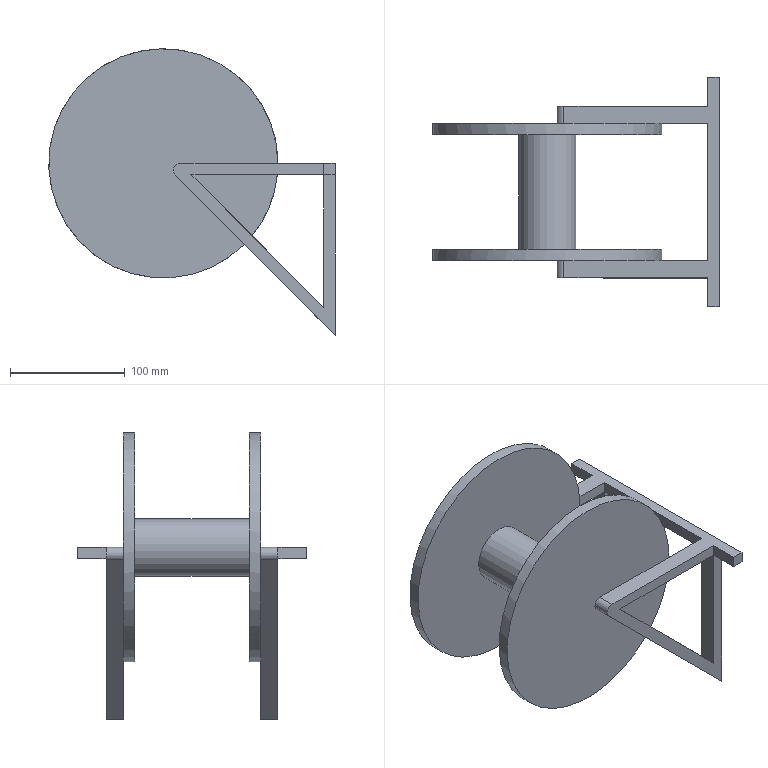Part | STEP file | daizhuantong | 1 solid | 35 faces | box 250 x 200 x 250 mm | volume 976487 mm3 | plane 30 | cylinder 5 | commonest cylinder face diameters 12 x2 200 x2 50 x1